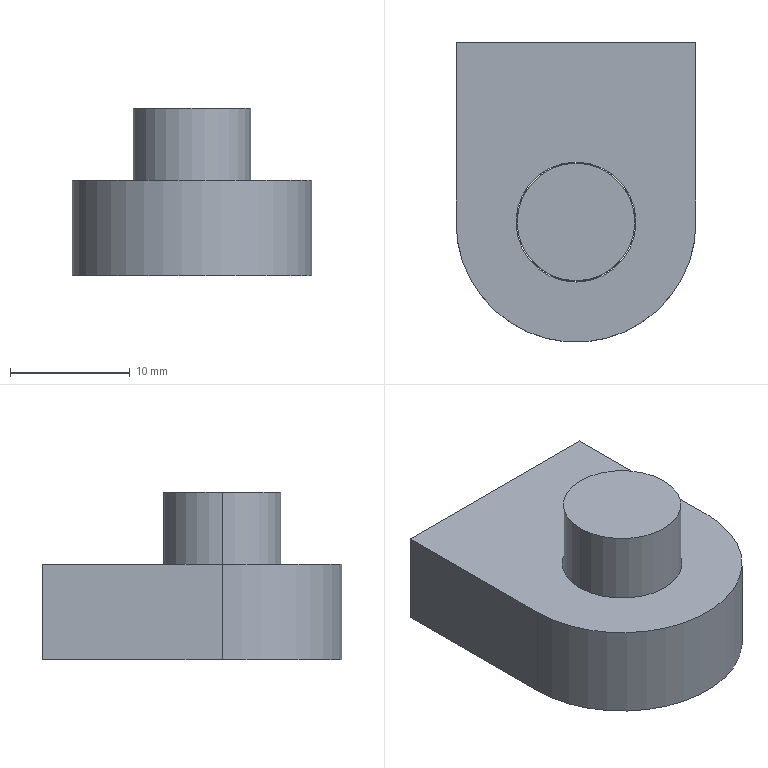Part | SolidWorks | features Extrusion 1, Revolution 1 | 2 solids | 12 faces | box 20 x 25 x 14 mm | volume 4084 mm3 | plane 7 | cylinder 5 | commonest cylinder face diameters 9.8 x2 10 x2 20 x1
STEP:
#1=CARTESIAN_POINT('',(-5.,0.,-8.));
#2=VERTEX_POINT('',#1);
#3=CARTESIAN_POINT('',(5.,0.,-8.));
#4=VERTEX_POINT('',#3);
#5=CARTESIAN_POINT('',(0.,0.,-8.));
#6=DIRECTION('',(0.,0.,1.));
#7=DIRECTION('',(1.,0.,0.));
#8=AXIS2_PLACEMENT_3D('',#5,#6,#7);
#9=CIRCLE('',#8,5.);
#10=EDGE_CURVE('',#2,#4,#9,.T.);
#11=ORIENTED_EDGE('',*,*,#10,.F.);
#12=CARTESIAN_POINT('',(-5.,0.,0.));
#13=VERTEX_POINT('',#12);
#14=CARTESIAN_POINT('',(-5.,0.,-8.));
#15=DIRECTION('',(0.,0.,1.));
#16=VECTOR('',#15,1000.);
#17=LINE('',#14,#16);
#18=EDGE_CURVE('',#2,#13,#17,.T.);
#19=ORIENTED_EDGE('',*,*,#18,.T.);
#20=CARTESIAN_POINT('',(5.,0.,0.));
#21=VERTEX_POINT('',#20);
#22=CARTESIAN_POINT('',(0.,0.,0.));
#23=DIRECTION('',(0.,0.,1.));
#24=DIRECTION('',(1.,0.,0.));
#25=AXIS2_PLACEMENT_3D('',#22,#23,#24);
#26=CIRCLE('',#25,5.);
#27=EDGE_CURVE('',#13,#21,#26,.T.);
#28=ORIENTED_EDGE('',*,*,#27,.T.);
#29=CARTESIAN_POINT('',(5.,0.,-8.));
#30=DIRECTION('',(0.,0.,1.));
#31=VECTOR('',#30,1000.);
#32=LINE('',#29,#31);
#33=EDGE_CURVE('',#4,#21,#32,.T.);
#34=ORIENTED_EDGE('',*,*,#33,.F.);
#35=EDGE_LOOP('',(#11,#19,#28,#34));
#36=FACE_OUTER_BOUND('',#35,.T.);
#37=CARTESIAN_POINT('',(0.,0.,-8.));
#38=DIRECTION('',(0.,0.,1.));
#39=DIRECTION('',(1.,0.,0.));
#40=AXIS2_PLACEMENT_3D('',#37,#38,#39);
#41=CYLINDRICAL_SURFACE('',#40,5.);
#42=ADVANCED_FACE('',(#36),#41,.F.);
#43=CARTESIAN_POINT('',(-10.,0.,0.));
#44=VERTEX_POINT('',#43);
#45=CARTESIAN_POINT('',(10.,0.,0.));
#46=VERTEX_POINT('',#45);
#47=CARTESIAN_POINT('',(0.,0.,0.));
#48=DIRECTION('',(0.,0.,1.));
#49=DIRECTION('',(1.,0.,0.));
#50=AXIS2_PLACEMENT_3D('',#47,#48,#49);
#51=CIRCLE('',#50,10.);
#52=EDGE_CURVE('',#44,#46,#51,.T.);
#53=ORIENTED_EDGE('',*,*,#52,.F.);
#54=CARTESIAN_POINT('',(-10.,0.,-8.));
#55=VERTEX_POINT('',#54);
#56=CARTESIAN_POINT('',(-10.,0.,-8.));
#57=DIRECTION('',(0.,0.,1.));
#58=VECTOR('',#57,1000.);
#59=LINE('',#56,#58);
#60=EDGE_CURVE('',#55,#44,#59,.T.);
#61=ORIENTED_EDGE('',*,*,#60,.F.);
#62=CARTESIAN_POINT('',(10.,0.,-8.));
#63=VERTEX_POINT('',#62);
#64=CARTESIAN_POINT('',(0.,0.,-8.));
#65=DIRECTION('',(0.,0.,1.));
#66=DIRECTION('',(1.,0.,0.));
#67=AXIS2_PLACEMENT_3D('',#64,#65,#66);
#68=CIRCLE('',#67,10.);
#69=EDGE_CURVE('',#55,#63,#68,.T.);
#70=ORIENTED_EDGE('',*,*,#69,.T.);
#71=CARTESIAN_POINT('',(10.,0.,-8.));
#72=DIRECTION('',(0.,0.,1.));
#73=VECTOR('',#72,1000.);
#74=LINE('',#71,#73);
#75=EDGE_CURVE('',#63,#46,#74,.T.);
#76=ORIENTED_EDGE('',*,*,#75,.T.);
#77=EDGE_LOOP('',(#53,#61,#70,#76));
#78=FACE_OUTER_BOUND('',#77,.T.);
#79=CARTESIAN_POINT('',(0.,0.,-8.));
#80=DIRECTION('',(0.,0.,1.));
#81=DIRECTION('',(1.,0.,0.));
#82=AXIS2_PLACEMENT_3D('',#79,#80,#81);
#83=CYLINDRICAL_SURFACE('',#82,10.);
#84=ADVANCED_FACE('',(#78),#83,.T.);
#85=CARTESIAN_POINT('',(-10.,15.,0.));
#86=VERTEX_POINT('',#85);
#87=CARTESIAN_POINT('',(-10.,15.,0.));
#88=DIRECTION('',(0.,-1.,0.));
#89=VECTOR('',#88,1000.);
#90=LINE('',#87,#89);
#91=EDGE_CURVE('',#86,#44,#90,.T.);
#92=ORIENTED_EDGE('',*,*,#91,.F.);
#93=CARTESIAN_POINT('',(-10.,15.,-8.));
#94=VERTEX_POINT('',#93);
#95=CARTESIAN_POINT('',(-10.,15.,-8.));
#96=DIRECTION('',(0.,0.,1.));
#97=VECTOR('',#96,1000.);
#98=LINE('',#95,#97);
#99=EDGE_CURVE('',#94,#86,#98,.T.);
#100=ORIENTED_EDGE('',*,*,#99,.F.);
#101=CARTESIAN_POINT('',(-10.,15.,-8.));
#102=DIRECTION('',(0.,-1.,0.));
#103=VECTOR('',#102,1000.);
#104=LINE('',#101,#103);
#105=EDGE_CURVE('',#94,#55,#104,.T.);
#106=ORIENTED_EDGE('',*,*,#105,.T.);
#107=ORIENTED_EDGE('',*,*,#60,.T.);
#108=EDGE_LOOP('',(#92,#100,#106,#107));
#109=FACE_OUTER_BOUND('',#108,.T.);
#110=CARTESIAN_POINT('',(-10.,15.,-8.));
#111=DIRECTION('',(-1.,0.,0.));
#112=DIRECTION('',(0.,0.,1.));
#113=AXIS2_PLACEMENT_3D('',#110,#111,#112);
#114=PLANE('',#113);
#115=ADVANCED_FACE('',(#109),#114,.T.);
#116=CARTESIAN_POINT('',(10.,15.,0.));
#117=VERTEX_POINT('',#116);
#118=CARTESIAN_POINT('',(10.,15.,0.));
#119=DIRECTION('',(-1.,0.,0.));
#120=VECTOR('',#119,1000.);
#121=LINE('',#118,#120);
#122=EDGE_CURVE('',#117,#86,#121,.T.);
#123=ORIENTED_EDGE('',*,*,#122,.F.);
#124=CARTESIAN_POINT('',(10.,15.,-8.));
#125=VERTEX_POINT('',#124);
#126=CARTESIAN_POINT('',(10.,15.,-8.));
#127=DIRECTION('',(0.,0.,1.));
#128=VECTOR('',#127,1000.);
#129=LINE('',#126,#128);
#130=EDGE_CURVE('',#125,#117,#129,.T.);
#131=ORIENTED_EDGE('',*,*,#130,.F.);
#132=CARTESIAN_POINT('',(10.,15.,-8.));
#133=DIRECTION('',(-1.,0.,0.));
#134=VECTOR('',#133,1000.);
#135=LINE('',#132,#134);
#136=EDGE_CURVE('',#125,#94,#135,.T.);
#137=ORIENTED_EDGE('',*,*,#136,.T.);
#138=ORIENTED_EDGE('',*,*,#99,.T.);
#139=EDGE_LOOP('',(#123,#131,#137,#138));
#140=FACE_OUTER_BOUND('',#139,.T.);
#141=CARTESIAN_POINT('',(10.,15.,-8.));
#142=DIRECTION('',(0.,1.,0.));
#143=DIRECTION('',(0.,0.,1.));
#144=AXIS2_PLACEMENT_3D('',#141,#142,#143);
#145=PLANE('',#144);
#146=ADVANCED_FACE('',(#140),#145,.T.);
#147=CARTESIAN_POINT('',(10.,0.,0.));
#148=DIRECTION('',(0.,1.,0.));
#149=VECTOR('',#148,1000.);
#150=LINE('',#147,#149);
#151=EDGE_CURVE('',#46,#117,#150,.T.);
#152=ORIENTED_EDGE('',*,*,#151,.F.);
#153=ORIENTED_EDGE('',*,*,#75,.F.);
#154=CARTESIAN_POINT('',(10.,0.,-8.));
#155=DIRECTION('',(0.,1.,0.));
#156=VECTOR('',#155,1000.);
#157=LINE('',#154,#156);
#158=EDGE_CURVE('',#63,#125,#157,.T.);
#159=ORIENTED_EDGE('',*,*,#158,.T.);
#160=ORIENTED_EDGE('',*,*,#130,.T.);
#161=EDGE_LOOP('',(#152,#153,#159,#160));
#162=FACE_OUTER_BOUND('',#161,.T.);
#163=CARTESIAN_POINT('',(10.,0.,-8.));
#164=DIRECTION('',(1.,0.,0.));
#165=DIRECTION('',(0.,0.,-1.));
#166=AXIS2_PLACEMENT_3D('',#163,#164,#165);
#167=PLANE('',#166);
#168=ADVANCED_FACE('',(#162),#167,.T.);
#169=CARTESIAN_POINT('',(0.,0.,-8.));
#170=DIRECTION('',(0.,0.,1.));
#171=DIRECTION('',(1.,0.,0.));
#172=AXIS2_PLACEMENT_3D('',#169,#170,#171);
#173=CIRCLE('',#172,5.);
#174=EDGE_CURVE('',#4,#2,#173,.T.);
#175=ORIENTED_EDGE('',*,*,#174,.T.);
#176=ORIENTED_EDGE('',*,*,#10,.T.);
#177=EDGE_LOOP('',(#175,#176));
#178=FACE_BOUND('',#177,.T.);
#179=ORIENTED_EDGE('',*,*,#69,.F.);
#180=ORIENTED_EDGE('',*,*,#105,.F.);
#181=ORIENTED_EDGE('',*,*,#136,.F.);
#182=ORIENTED_EDGE('',*,*,#158,.F.);
#183=EDGE_LOOP('',(#179,#180,#181,#182));
#184=FACE_OUTER_BOUND('',#183,.T.);
#185=CARTESIAN_POINT('',(0.,0.,-8.));
#186=DIRECTION('',(0.,0.,1.));
#187=DIRECTION('',(1.,0.,0.));
#188=AXIS2_PLACEMENT_3D('',#185,#186,#187);
#189=PLANE('',#188);
#190=ADVANCED_FACE('',(#178,#184),#189,.F.);
#191=CARTESIAN_POINT('',(0.,0.,0.));
#192=DIRECTION('',(0.,0.,1.));
#193=DIRECTION('',(1.,0.,0.));
#194=AXIS2_PLACEMENT_3D('',#191,#192,#193);
#195=CIRCLE('',#194,5.);
#196=EDGE_CURVE('',#21,#13,#195,.T.);
#197=ORIENTED_EDGE('',*,*,#196,.F.);
#198=ORIENTED_EDGE('',*,*,#27,.F.);
#199=EDGE_LOOP('',(#197,#198));
#200=FACE_BOUND('',#199,.T.);
#201=ORIENTED_EDGE('',*,*,#52,.T.);
#202=ORIENTED_EDGE('',*,*,#151,.T.);
#203=ORIENTED_EDGE('',*,*,#122,.T.);
#204=ORIENTED_EDGE('',*,*,#91,.T.);
#205=EDGE_LOOP('',(#201,#202,#203,#204));
#206=FACE_OUTER_BOUND('',#205,.T.);
#207=CARTESIAN_POINT('',(0.,0.,0.));
#208=DIRECTION('',(0.,0.,1.));
#209=DIRECTION('',(1.,0.,0.));
#210=AXIS2_PLACEMENT_3D('',#207,#208,#209);
#211=PLANE('',#210);
#212=ADVANCED_FACE('',(#200,#206),#211,.T.);
#213=ORIENTED_EDGE('',*,*,#18,.F.);
#214=ORIENTED_EDGE('',*,*,#174,.F.);
#215=ORIENTED_EDGE('',*,*,#33,.T.);
#216=ORIENTED_EDGE('',*,*,#196,.T.);
#217=EDGE_LOOP('',(#213,#214,#215,#216));
#218=FACE_OUTER_BOUND('',#217,.T.);
#219=CARTESIAN_POINT('',(0.,0.,-8.));
#220=DIRECTION('',(0.,0.,1.));
#221=DIRECTION('',(1.,0.,0.));
#222=AXIS2_PLACEMENT_3D('',#219,#220,#221);
#223=CYLINDRICAL_SURFACE('',#222,5.);
#224=ADVANCED_FACE('',(#218),#223,.F.);
#225=CLOSED_SHELL('',(#42,#84,#115,#146,#168,#190,#212,#224));
#226=MANIFOLD_SOLID_BREP('',#225);
#227=CARTESIAN_POINT('',(4.9,0.,-8.));
#228=VERTEX_POINT('',#227);
#229=CARTESIAN_POINT('',(-4.9,0.,-8.));
#230=VERTEX_POINT('',#229);
#231=CARTESIAN_POINT('',(0.,0.,-8.));
#232=DIRECTION('',(0.,0.,1.));
#233=DIRECTION('',(1.,0.,0.));
#234=AXIS2_PLACEMENT_3D('',#231,#232,#233);
#235=CIRCLE('',#234,4.9);
#236=EDGE_CURVE('',#228,#230,#235,.T.);
#237=ORIENTED_EDGE('',*,*,#236,.T.);
#238=CARTESIAN_POINT('',(-4.9,0.,6.));
#239=VERTEX_POINT('',#238);
#240=CARTESIAN_POINT('',(-4.9,0.,-8.));
#241=DIRECTION('',(0.,0.,1.));
#242=VECTOR('',#241,1000.);
#243=LINE('',#240,#242);
#244=EDGE_CURVE('',#230,#239,#243,.T.);
#245=ORIENTED_EDGE('',*,*,#244,.T.);
#246=CARTESIAN_POINT('',(4.9,0.,6.));
#247=VERTEX_POINT('',#246);
#248=CARTESIAN_POINT('',(0.,0.,6.));
#249=DIRECTION('',(0.,0.,1.));
#250=DIRECTION('',(1.,0.,0.));
#251=AXIS2_PLACEMENT_3D('',#248,#249,#250);
#252=CIRCLE('',#251,4.9);
#253=EDGE_CURVE('',#247,#239,#252,.T.);
#254=ORIENTED_EDGE('',*,*,#253,.F.);
#255=CARTESIAN_POINT('',(4.9,0.,-8.));
#256=DIRECTION('',(0.,0.,1.));
#257=VECTOR('',#256,1000.);
#258=LINE('',#255,#257);
#259=EDGE_CURVE('',#228,#247,#258,.T.);
#260=ORIENTED_EDGE('',*,*,#259,.F.);
#261=EDGE_LOOP('',(#237,#245,#254,#260));
#262=FACE_OUTER_BOUND('',#261,.T.);
#263=CARTESIAN_POINT('',(0.,0.,-8.));
#264=DIRECTION('',(0.,0.,1.));
#265=DIRECTION('',(1.,0.,0.));
#266=AXIS2_PLACEMENT_3D('',#263,#264,#265);
#267=CYLINDRICAL_SURFACE('',#266,4.9);
#268=ADVANCED_FACE('',(#262),#267,.T.);
#269=ORIENTED_EDGE('',*,*,#244,.F.);
#270=CARTESIAN_POINT('',(0.,0.,-8.));
#271=DIRECTION('',(0.,0.,1.));
#272=DIRECTION('',(1.,0.,0.));
#273=AXIS2_PLACEMENT_3D('',#270,#271,#272);
#274=CIRCLE('',#273,4.9);
#275=EDGE_CURVE('',#230,#228,#274,.T.);
#276=ORIENTED_EDGE('',*,*,#275,.T.);
#277=ORIENTED_EDGE('',*,*,#259,.T.);
#278=CARTESIAN_POINT('',(0.,0.,6.));
#279=DIRECTION('',(0.,0.,1.));
#280=DIRECTION('',(1.,0.,0.));
#281=AXIS2_PLACEMENT_3D('',#278,#279,#280);
#282=CIRCLE('',#281,4.9);
#283=EDGE_CURVE('',#239,#247,#282,.T.);
#284=ORIENTED_EDGE('',*,*,#283,.F.);
#285=EDGE_LOOP('',(#269,#276,#277,#284));
#286=FACE_OUTER_BOUND('',#285,.T.);
#287=CARTESIAN_POINT('',(0.,0.,-8.));
#288=DIRECTION('',(0.,0.,1.));
#289=DIRECTION('',(1.,0.,0.));
#290=AXIS2_PLACEMENT_3D('',#287,#288,#289);
#291=CYLINDRICAL_SURFACE('',#290,4.9);
#292=ADVANCED_FACE('',(#286),#291,.T.);
#293=ORIENTED_EDGE('',*,*,#236,.F.);
#294=ORIENTED_EDGE('',*,*,#275,.F.);
#295=EDGE_LOOP('',(#293,#294));
#296=FACE_OUTER_BOUND('',#295,.T.);
#297=CARTESIAN_POINT('',(4.9,0.,-8.));
#298=DIRECTION('',(0.,0.,-1.));
#299=DIRECTION('',(-1.,0.,0.));
#300=AXIS2_PLACEMENT_3D('',#297,#298,#299);
#301=PLANE('',#300);
#302=ADVANCED_FACE('',(#296),#301,.T.);
#303=ORIENTED_EDGE('',*,*,#253,.T.);
#304=ORIENTED_EDGE('',*,*,#283,.T.);
#305=EDGE_LOOP('',(#303,#304));
#306=FACE_OUTER_BOUND('',#305,.T.);
#307=CARTESIAN_POINT('',(0.,0.,6.));
#308=DIRECTION('',(0.,0.,1.));
#309=DIRECTION('',(1.,0.,0.));
#310=AXIS2_PLACEMENT_3D('',#307,#308,#309);
#311=PLANE('',#310);
#312=ADVANCED_FACE('',(#306),#311,.T.);
#313=CLOSED_SHELL('',(#268,#292,#302,#312));
#314=MANIFOLD_SOLID_BREP('',#313);
#315=CARTESIAN_POINT('',(0.,0.,0.));
#316=DIRECTION('',(0.,0.,1.));
#317=DIRECTION('',(1.,0.,0.));
#318=AXIS2_PLACEMENT_3D('',#315,#316,#317);
#319=(LENGTH_UNIT()NAMED_UNIT(*)SI_UNIT(.MILLI.,.METRE.));
#320=UNCERTAINTY_MEASURE_WITH_UNIT(LENGTH_MEASURE(0.00001),#319,'','');
#321=(NAMED_UNIT(*)PLANE_ANGLE_UNIT()SI_UNIT($,.RADIAN.));
#322=(NAMED_UNIT(*)SI_UNIT($,.STERADIAN.)SOLID_ANGLE_UNIT());
#323=(GEOMETRIC_REPRESENTATION_CONTEXT(3)GLOBAL_UNCERTAINTY_ASSIGNED_CONTEXT((#320))GLOBAL_UNIT_ASSIGNED_CONTEXT((#319,#321,#322))REPRESENTATION_CONTEXT('',''));
#324=ADVANCED_BREP_SHAPE_REPRESENTATION('',(#226,#314,#318),#323);